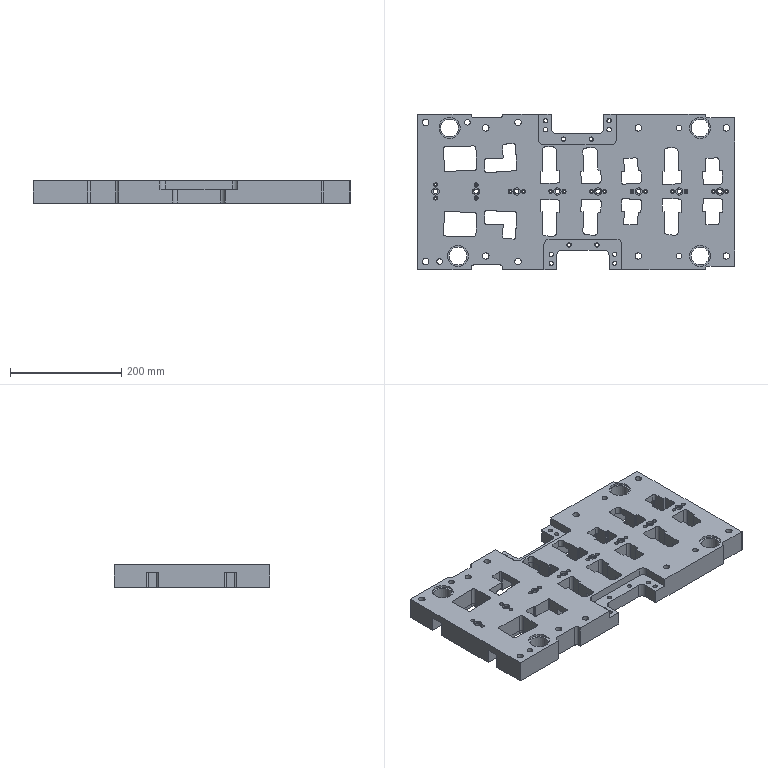Part | NX | features PS-15 2 | 1 solid | 520 faces | box 570 x 280 x 40 mm | volume 4293357 mm3 | cylinder 262 | plane 250 | cone 8 | commonest cylinder face diameters 8 x45 10 x26 6 x19 18 x18 4.001 x16 7 x16